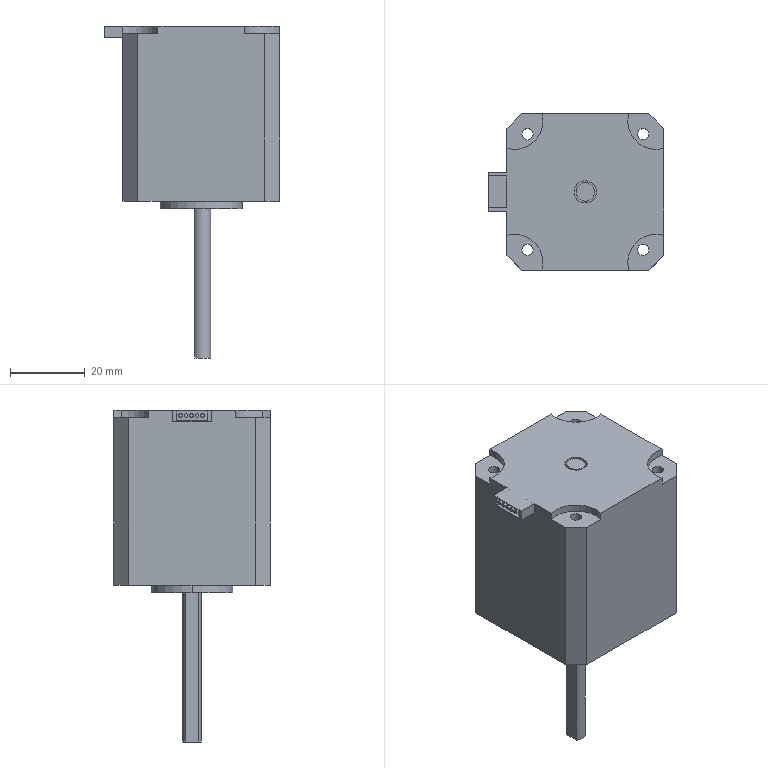Part | SolidWorks | features ICE 8, Extrusion 1 | 1 solid | 65 faces | box 47 x 42 x 89 mm | volume 81069 mm3 | plane 33 | cylinder 32 | commonest cylinder face diameters 1 x10 3 x8 15.282 x6 5 x4 6 x2 22 x2